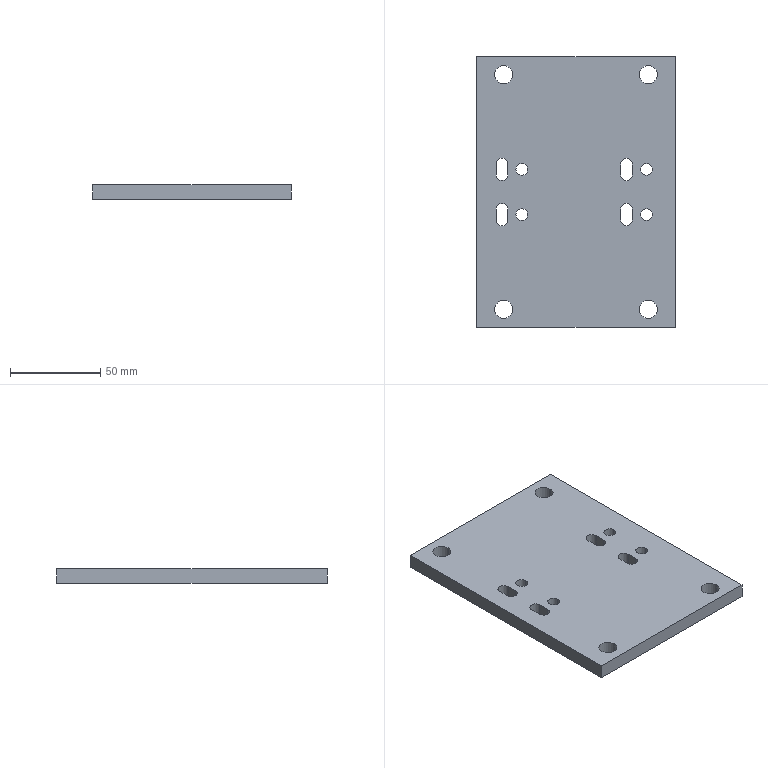Part | STEP file | vibratory feeder support plate | 1 solid | 38 faces | box 110 x 150 x 8 mm | volume 126115 mm3 | cylinder 24 | plane 14 | commonest cylinder face diameters 6.5 x16 10 x8